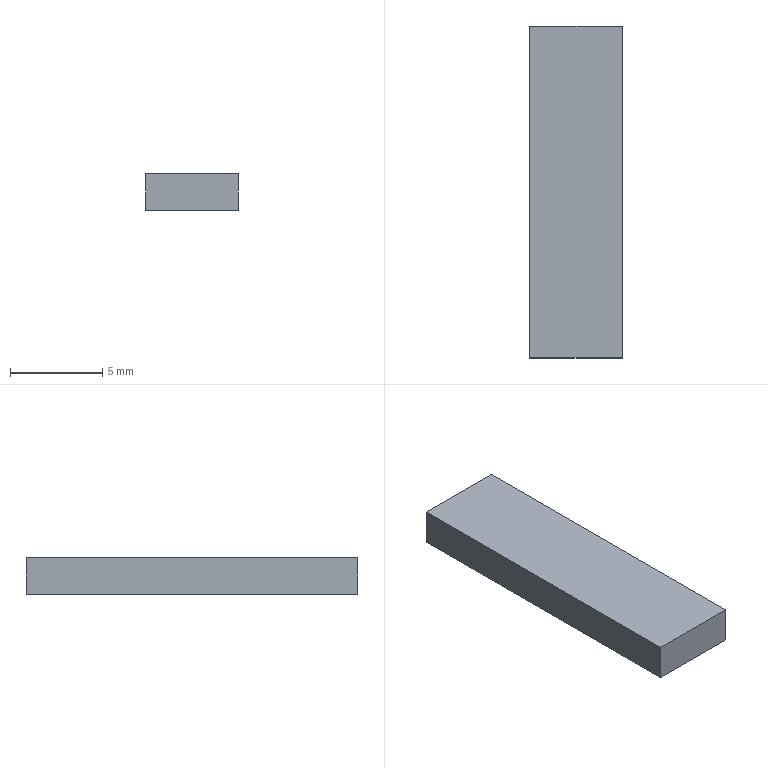Part | NX | features DATUM_CSYS 2, EXTRUDE 1, SKETCH 1 | 1 solid | 6 faces | box 5 x 18 x 2 mm | volume 180 mm3 | plane 6
STEP:
#1=CARTESIAN_POINT('',(-5.186,5.762,0.));
#2=VERTEX_POINT('',#1);
#3=CARTESIAN_POINT('',(-5.186,-12.238,0.));
#4=VERTEX_POINT('',#3);
#5=CARTESIAN_POINT('',(-5.186,5.762,0.));
#6=DIRECTION('',(0.,-1.,0.));
#7=VECTOR('',#6,1000.);
#8=LINE('',#5,#7);
#9=EDGE_CURVE('',#2,#4,#8,.T.);
#10=ORIENTED_EDGE('',*,*,#9,.T.);
#11=CARTESIAN_POINT('',(-5.186,-12.238,2.));
#12=VERTEX_POINT('',#11);
#13=CARTESIAN_POINT('',(-5.186,-12.238,2.));
#14=DIRECTION('',(0.,0.,-1.));
#15=VECTOR('',#14,1000.);
#16=LINE('',#13,#15);
#17=EDGE_CURVE('',#12,#4,#16,.T.);
#18=ORIENTED_EDGE('',*,*,#17,.F.);
#19=CARTESIAN_POINT('',(-5.186,5.762,2.));
#20=VERTEX_POINT('',#19);
#21=CARTESIAN_POINT('',(-5.186,5.762,2.));
#22=DIRECTION('',(0.,-1.,0.));
#23=VECTOR('',#22,1000.);
#24=LINE('',#21,#23);
#25=EDGE_CURVE('',#20,#12,#24,.T.);
#26=ORIENTED_EDGE('',*,*,#25,.F.);
#27=CARTESIAN_POINT('',(-5.186,5.762,2.));
#28=DIRECTION('',(0.,0.,-1.));
#29=VECTOR('',#28,1000.);
#30=LINE('',#27,#29);
#31=EDGE_CURVE('',#20,#2,#30,.T.);
#32=ORIENTED_EDGE('',*,*,#31,.T.);
#33=EDGE_LOOP('',(#10,#18,#26,#32));
#34=FACE_BOUND('',#33,.T.);
#35=CARTESIAN_POINT('',(-5.186,5.762,2.));
#36=DIRECTION('',(1.,0.,0.));
#37=DIRECTION('',(0.,0.,-1.));
#38=AXIS2_PLACEMENT_3D('',#35,#36,#37);
#39=PLANE('',#38);
#40=ADVANCED_FACE('',(#34),#39,.F.);
#41=CARTESIAN_POINT('',(-0.1864,-12.238,0.));
#42=VERTEX_POINT('',#41);
#43=CARTESIAN_POINT('',(-5.186,-12.238,0.));
#44=DIRECTION('',(1.,0.,0.));
#45=VECTOR('',#44,1000.);
#46=LINE('',#43,#45);
#47=EDGE_CURVE('',#4,#42,#46,.T.);
#48=ORIENTED_EDGE('',*,*,#47,.T.);
#49=CARTESIAN_POINT('',(-0.1864,-12.238,2.));
#50=VERTEX_POINT('',#49);
#51=CARTESIAN_POINT('',(-0.1864,-12.238,2.));
#52=DIRECTION('',(0.,0.,-1.));
#53=VECTOR('',#52,1000.);
#54=LINE('',#51,#53);
#55=EDGE_CURVE('',#50,#42,#54,.T.);
#56=ORIENTED_EDGE('',*,*,#55,.F.);
#57=CARTESIAN_POINT('',(-5.186,-12.238,2.));
#58=DIRECTION('',(1.,0.,0.));
#59=VECTOR('',#58,1000.);
#60=LINE('',#57,#59);
#61=EDGE_CURVE('',#12,#50,#60,.T.);
#62=ORIENTED_EDGE('',*,*,#61,.F.);
#63=ORIENTED_EDGE('',*,*,#17,.T.);
#64=EDGE_LOOP('',(#48,#56,#62,#63));
#65=FACE_BOUND('',#64,.T.);
#66=CARTESIAN_POINT('',(-5.186,-12.238,2.));
#67=DIRECTION('',(0.,1.,0.));
#68=DIRECTION('',(-1.,0.,0.));
#69=AXIS2_PLACEMENT_3D('',#66,#67,#68);
#70=PLANE('',#69);
#71=ADVANCED_FACE('',(#65),#70,.F.);
#72=CARTESIAN_POINT('',(-0.1864,5.762,0.));
#73=VERTEX_POINT('',#72);
#74=CARTESIAN_POINT('',(-0.1864,-12.238,0.));
#75=DIRECTION('',(0.,1.,0.));
#76=VECTOR('',#75,1000.);
#77=LINE('',#74,#76);
#78=EDGE_CURVE('',#42,#73,#77,.T.);
#79=ORIENTED_EDGE('',*,*,#78,.T.);
#80=CARTESIAN_POINT('',(-0.1864,5.762,2.));
#81=VERTEX_POINT('',#80);
#82=CARTESIAN_POINT('',(-0.1864,5.762,2.));
#83=DIRECTION('',(0.,0.,-1.));
#84=VECTOR('',#83,1000.);
#85=LINE('',#82,#84);
#86=EDGE_CURVE('',#81,#73,#85,.T.);
#87=ORIENTED_EDGE('',*,*,#86,.F.);
#88=CARTESIAN_POINT('',(-0.1864,-12.238,2.));
#89=DIRECTION('',(0.,1.,0.));
#90=VECTOR('',#89,1000.);
#91=LINE('',#88,#90);
#92=EDGE_CURVE('',#50,#81,#91,.T.);
#93=ORIENTED_EDGE('',*,*,#92,.F.);
#94=ORIENTED_EDGE('',*,*,#55,.T.);
#95=EDGE_LOOP('',(#79,#87,#93,#94));
#96=FACE_BOUND('',#95,.T.);
#97=CARTESIAN_POINT('',(-0.1864,-12.238,2.));
#98=DIRECTION('',(-1.,0.,0.));
#99=DIRECTION('',(0.,-1.,0.));
#100=AXIS2_PLACEMENT_3D('',#97,#98,#99);
#101=PLANE('',#100);
#102=ADVANCED_FACE('',(#96),#101,.F.);
#103=CARTESIAN_POINT('',(-0.1864,5.762,0.));
#104=DIRECTION('',(-1.,0.,0.));
#105=VECTOR('',#104,1000.);
#106=LINE('',#103,#105);
#107=EDGE_CURVE('',#73,#2,#106,.T.);
#108=ORIENTED_EDGE('',*,*,#107,.T.);
#109=ORIENTED_EDGE('',*,*,#31,.F.);
#110=CARTESIAN_POINT('',(-0.1864,5.762,2.));
#111=DIRECTION('',(-1.,0.,0.));
#112=VECTOR('',#111,1000.);
#113=LINE('',#110,#112);
#114=EDGE_CURVE('',#81,#20,#113,.T.);
#115=ORIENTED_EDGE('',*,*,#114,.F.);
#116=ORIENTED_EDGE('',*,*,#86,.T.);
#117=EDGE_LOOP('',(#108,#109,#115,#116));
#118=FACE_BOUND('',#117,.T.);
#119=CARTESIAN_POINT('',(-0.1864,5.762,2.));
#120=DIRECTION('',(0.,-1.,0.));
#121=DIRECTION('',(1.,0.,0.));
#122=AXIS2_PLACEMENT_3D('',#119,#120,#121);
#123=PLANE('',#122);
#124=ADVANCED_FACE('',(#118),#123,.F.);
#125=ORIENTED_EDGE('',*,*,#25,.T.);
#126=ORIENTED_EDGE('',*,*,#61,.T.);
#127=ORIENTED_EDGE('',*,*,#92,.T.);
#128=ORIENTED_EDGE('',*,*,#114,.T.);
#129=EDGE_LOOP('',(#125,#126,#127,#128));
#130=FACE_BOUND('',#129,.T.);
#131=CARTESIAN_POINT('',(0.,0.,2.));
#132=DIRECTION('',(0.,0.,1.));
#133=DIRECTION('',(1.,0.,0.));
#134=AXIS2_PLACEMENT_3D('',#131,#132,#133);
#135=PLANE('',#134);
#136=ADVANCED_FACE('',(#130),#135,.T.);
#137=ORIENTED_EDGE('',*,*,#9,.F.);
#138=ORIENTED_EDGE('',*,*,#107,.F.);
#139=ORIENTED_EDGE('',*,*,#78,.F.);
#140=ORIENTED_EDGE('',*,*,#47,.F.);
#141=EDGE_LOOP('',(#137,#138,#139,#140));
#142=FACE_BOUND('',#141,.T.);
#143=CARTESIAN_POINT('',(0.,0.,0.));
#144=DIRECTION('',(0.,0.,1.));
#145=DIRECTION('',(1.,0.,0.));
#146=AXIS2_PLACEMENT_3D('',#143,#144,#145);
#147=PLANE('',#146);
#148=ADVANCED_FACE('',(#142),#147,.F.);
#149=CLOSED_SHELL('',(#40,#71,#102,#124,#136,#148));
#150=MANIFOLD_SOLID_BREP('',#149);
#151=(LENGTH_UNIT()NAMED_UNIT(*)SI_UNIT(.MILLI.,.METRE.));
#152=UNCERTAINTY_MEASURE_WITH_UNIT(LENGTH_MEASURE(0.00001),#151,'','');
#153=(NAMED_UNIT(*)PLANE_ANGLE_UNIT()SI_UNIT($,.RADIAN.));
#154=(NAMED_UNIT(*)SI_UNIT($,.STERADIAN.)SOLID_ANGLE_UNIT());
#155=(GEOMETRIC_REPRESENTATION_CONTEXT(3)GLOBAL_UNCERTAINTY_ASSIGNED_CONTEXT((#152))GLOBAL_UNIT_ASSIGNED_CONTEXT((#151,#153,#154))REPRESENTATION_CONTEXT('',''));
#156=ADVANCED_BREP_SHAPE_REPRESENTATION('',(#150),#155);